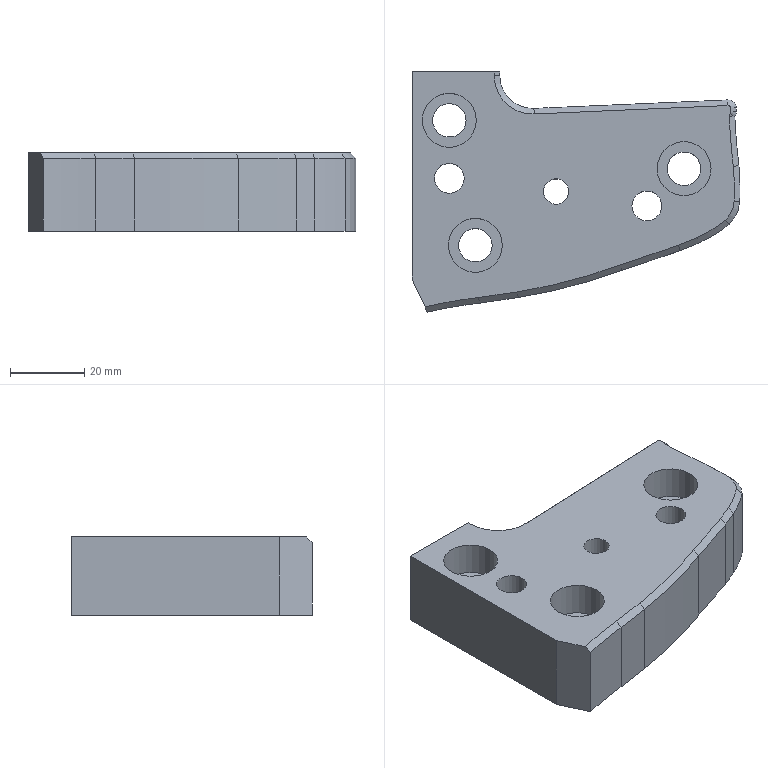Part | NX | features 23 2 | 1 solid | 48 faces | box 88.04 x 64.484 x 21 mm | volume 80340 mm3 | cylinder 20 | plane 16 | cone 12 | commonest cylinder face diameters 9 x3 14.5 x3 4.4 x2 8.001 x2 6.8 x1 17.6 x1
STEP:
#1=CARTESIAN_POINT('',(1059.999,248.439,-23.5));
#2=VERTEX_POINT('',#1);
#3=CARTESIAN_POINT('',(1064.,248.439,-23.5));
#4=DIRECTION('',(0.,0.,1.));
#5=DIRECTION('',(-1.,0.,0.));
#6=AXIS2_PLACEMENT_3D('',#3,#4,#5);
#7=CIRCLE('',#6,4.);
#8=EDGE_CURVE('',#2,#2,#7,.T.);
#9=ORIENTED_EDGE('',*,*,#8,.T.);
#10=EDGE_LOOP('',(#9));
#11=FACE_BOUND('',#10,.T.);
#12=CARTESIAN_POINT('',(1059.5,264.,-23.5));
#13=VERTEX_POINT('',#12);
#14=CARTESIAN_POINT('',(1064.,264.,-23.5));
#15=DIRECTION('',(0.,0.,1.));
#16=DIRECTION('',(-1.,0.,0.));
#17=AXIS2_PLACEMENT_3D('',#14,#15,#16);
#18=CIRCLE('',#17,4.5);
#19=EDGE_CURVE('',#13,#13,#18,.T.);
#20=ORIENTED_EDGE('',*,*,#19,.T.);
#21=EDGE_LOOP('',(#20));
#22=FACE_BOUND('',#21,.T.);
#23=CARTESIAN_POINT('',(1122.54,251.,-23.5));
#24=VERTEX_POINT('',#23);
#25=CARTESIAN_POINT('',(1127.04,251.,-23.5));
#26=DIRECTION('',(0.,0.,1.));
#27=DIRECTION('',(-1.,0.,0.));
#28=AXIS2_PLACEMENT_3D('',#25,#26,#27);
#29=CIRCLE('',#28,4.5);
#30=EDGE_CURVE('',#24,#24,#29,.T.);
#31=ORIENTED_EDGE('',*,*,#30,.T.);
#32=EDGE_LOOP('',(#31));
#33=FACE_BOUND('',#32,.T.);
#34=CARTESIAN_POINT('',(1066.5,230.439,-23.5));
#35=VERTEX_POINT('',#34);
#36=CARTESIAN_POINT('',(1071.,230.439,-23.5));
#37=DIRECTION('',(0.,0.,1.));
#38=DIRECTION('',(-1.,0.,0.));
#39=AXIS2_PLACEMENT_3D('',#36,#37,#38);
#40=CIRCLE('',#39,4.5);
#41=EDGE_CURVE('',#35,#35,#40,.T.);
#42=ORIENTED_EDGE('',*,*,#41,.T.);
#43=EDGE_LOOP('',(#42));
#44=FACE_BOUND('',#43,.T.);
#45=CARTESIAN_POINT('',(1113.04,241.,-23.5));
#46=VERTEX_POINT('',#45);
#47=CARTESIAN_POINT('',(1117.04,241.,-23.5));
#48=DIRECTION('',(0.,0.,1.));
#49=DIRECTION('',(-1.,0.,0.));
#50=AXIS2_PLACEMENT_3D('',#47,#48,#49);
#51=CIRCLE('',#50,4.);
#52=EDGE_CURVE('',#46,#46,#51,.T.);
#53=ORIENTED_EDGE('',*,*,#52,.T.);
#54=EDGE_LOOP('',(#53));
#55=FACE_BOUND('',#54,.T.);
#56=CARTESIAN_POINT('',(1089.301,244.877,-23.5));
#57=VERTEX_POINT('',#56);
#58=CARTESIAN_POINT('',(1092.701,244.877,-23.5));
#59=DIRECTION('',(0.,0.,1.));
#60=DIRECTION('',(-1.,0.,0.));
#61=AXIS2_PLACEMENT_3D('',#58,#59,#60);
#62=CIRCLE('',#61,3.4);
#63=EDGE_CURVE('',#57,#57,#62,.T.);
#64=ORIENTED_EDGE('',*,*,#63,.T.);
#65=EDGE_LOOP('',(#64));
#66=FACE_BOUND('',#65,.T.);
#67=CARTESIAN_POINT('',(1058.121,212.516,-23.5));
#68=VERTEX_POINT('',#67);
#69=CARTESIAN_POINT('',(1072.065,214.923,-23.5));
#70=VERTEX_POINT('',#69);
#71=CARTESIAN_POINT('',(1086.33,90.693,-23.5));
#72=DIRECTION('',(0.,0.,-1.));
#73=DIRECTION('',(-1.,0.,0.));
#74=AXIS2_PLACEMENT_3D('',#71,#72,#73);
#75=CIRCLE('',#74,125.047);
#76=EDGE_CURVE('',#68,#70,#75,.T.);
#77=ORIENTED_EDGE('',*,*,#76,.F.);
#78=CARTESIAN_POINT('',(1054.,221.377,-23.5));
#79=VERTEX_POINT('',#78);
#80=CARTESIAN_POINT('',(1052.952,223.63,-23.5));
#81=DIRECTION('',(0.4218,-0.9067,0.));
#82=VECTOR('',#81,1000.);
#83=LINE('',#80,#82);
#84=EDGE_CURVE('',#79,#68,#83,.T.);
#85=ORIENTED_EDGE('',*,*,#84,.F.);
#86=CARTESIAN_POINT('',(1054.,277.,-23.5));
#87=VERTEX_POINT('',#86);
#88=CARTESIAN_POINT('',(1054.,328.5,-23.5));
#89=DIRECTION('',(0.,1.,0.));
#90=VECTOR('',#89,1000.);
#91=LINE('',#88,#90);
#92=EDGE_CURVE('',#79,#87,#91,.T.);
#93=ORIENTED_EDGE('',*,*,#92,.T.);
#94=CARTESIAN_POINT('',(1077.541,277.,-23.5));
#95=VERTEX_POINT('',#94);
#96=CARTESIAN_POINT('',(1136.,277.,-23.5));
#97=DIRECTION('',(1.,0.,0.));
#98=VECTOR('',#97,1000.);
#99=LINE('',#96,#98);
#100=EDGE_CURVE('',#87,#95,#99,.T.);
#101=ORIENTED_EDGE('',*,*,#100,.T.);
#102=CARTESIAN_POINT('',(1077.541,275.983,-23.5));
#103=VERTEX_POINT('',#102);
#104=CARTESIAN_POINT('',(1077.541,328.5,-23.5));
#105=DIRECTION('',(0.,-1.,0.));
#106=VECTOR('',#105,1000.);
#107=LINE('',#104,#106);
#108=EDGE_CURVE('',#95,#103,#107,.T.);
#109=ORIENTED_EDGE('',*,*,#108,.T.);
#110=CARTESIAN_POINT('',(1086.725,267.191,-23.5));
#111=VERTEX_POINT('',#110);
#112=CARTESIAN_POINT('',(1086.341,275.983,-23.5));
#113=DIRECTION('',(0.,0.,1.));
#114=DIRECTION('',(-1.,0.,0.));
#115=AXIS2_PLACEMENT_3D('',#112,#113,#114);
#116=CIRCLE('',#115,8.8);
#117=EDGE_CURVE('',#103,#111,#116,.T.);
#118=ORIENTED_EDGE('',*,*,#117,.T.);
#119=CARTESIAN_POINT('',(1138.773,269.461,-23.5));
#120=VERTEX_POINT('',#119);
#121=CARTESIAN_POINT('',(1138.575,269.452,-23.5));
#122=DIRECTION('',(0.9991,0.04356,0.));
#123=VECTOR('',#122,1000.);
#124=LINE('',#121,#123);
#125=EDGE_CURVE('',#111,#120,#124,.T.);
#126=ORIENTED_EDGE('',*,*,#125,.T.);
#127=CARTESIAN_POINT('',(1141.067,267.339,-23.5));
#128=VERTEX_POINT('',#127);
#129=CARTESIAN_POINT('',(1138.868,267.263,-23.5));
#130=DIRECTION('',(0.,0.,1.));
#131=DIRECTION('',(-1.,0.,0.));
#132=AXIS2_PLACEMENT_3D('',#129,#130,#131);
#133=CIRCLE('',#132,2.2);
#134=EDGE_CURVE('',#128,#120,#133,.T.);
#135=ORIENTED_EDGE('',*,*,#134,.F.);
#136=CARTESIAN_POINT('',(1141.104,266.344,-23.5));
#137=VERTEX_POINT('',#136);
#138=CARTESIAN_POINT('',(1326.856,273.811,-23.5));
#139=DIRECTION('',(0.,0.,1.));
#140=DIRECTION('',(-1.,0.,0.));
#141=AXIS2_PLACEMENT_3D('',#138,#139,#140);
#142=CIRCLE('',#141,185.901);
#143=EDGE_CURVE('',#128,#137,#142,.T.);
#144=ORIENTED_EDGE('',*,*,#143,.T.);
#145=CARTESIAN_POINT('',(1140.666,264.943,-23.5));
#146=VERTEX_POINT('',#145);
#147=CARTESIAN_POINT('',(1138.906,266.263,-23.5));
#148=DIRECTION('',(0.,0.,1.));
#149=DIRECTION('',(-1.,0.,0.));
#150=AXIS2_PLACEMENT_3D('',#147,#148,#149);
#151=CIRCLE('',#150,2.2);
#152=EDGE_CURVE('',#146,#137,#151,.T.);
#153=ORIENTED_EDGE('',*,*,#152,.F.);
#154=CARTESIAN_POINT('',(1141.757,251.812,-23.5));
#155=VERTEX_POINT('',#154);
#156=CARTESIAN_POINT('',(1326.856,273.811,-23.5));
#157=DIRECTION('',(0.,0.,1.));
#158=DIRECTION('',(-1.,0.,0.));
#159=AXIS2_PLACEMENT_3D('',#156,#157,#158);
#160=CIRCLE('',#159,186.401);
#161=EDGE_CURVE('',#146,#155,#160,.T.);
#162=ORIENTED_EDGE('',*,*,#161,.T.);
#163=CARTESIAN_POINT('',(1141.998,242.228,-23.5));
#164=VERTEX_POINT('',#163);
#165=CARTESIAN_POINT('',(1057.602,244.9,-23.5));
#166=DIRECTION('',(0.,0.,-1.));
#167=DIRECTION('',(-1.,0.,0.));
#168=AXIS2_PLACEMENT_3D('',#165,#166,#167);
#169=CIRCLE('',#168,84.438);
#170=EDGE_CURVE('',#155,#164,#169,.T.);
#171=ORIENTED_EDGE('',*,*,#170,.T.);
#172=CARTESIAN_POINT('',(1139.107,236.023,-23.5));
#173=VERTEX_POINT('',#172);
#174=CARTESIAN_POINT('',(1132.519,242.868,-23.5));
#175=DIRECTION('',(0.,0.,1.));
#176=DIRECTION('',(-1.,0.,0.));
#177=AXIS2_PLACEMENT_3D('',#174,#175,#176);
#178=CIRCLE('',#177,9.5);
#179=EDGE_CURVE('',#173,#164,#178,.T.);
#180=ORIENTED_EDGE('',*,*,#179,.F.);
#181=CARTESIAN_POINT('',(1131.001,231.048,-23.5));
#182=VERTEX_POINT('',#181);
#183=CARTESIAN_POINT('',(1115.023,266.175,-23.5));
#184=DIRECTION('',(0.,0.,-1.));
#185=DIRECTION('',(-1.,0.,0.));
#186=AXIS2_PLACEMENT_3D('',#183,#184,#185);
#187=CIRCLE('',#186,38.59);
#188=EDGE_CURVE('',#173,#182,#187,.T.);
#189=ORIENTED_EDGE('',*,*,#188,.T.);
#190=CARTESIAN_POINT('',(1126.024,229.046,-23.5));
#191=VERTEX_POINT('',#190);
#192=CARTESIAN_POINT('',(1169.044,246.35,-23.5));
#193=DIRECTION('',(0.9278,0.3732,0.));
#194=VECTOR('',#193,1000.);
#195=LINE('',#192,#194);
#196=EDGE_CURVE('',#191,#182,#195,.T.);
#197=ORIENTED_EDGE('',*,*,#196,.F.);
#198=CARTESIAN_POINT('',(1110.455,223.763,-23.5));
#199=VERTEX_POINT('',#198);
#200=CARTESIAN_POINT('',(597.176,1761.975,-23.5));
#201=DIRECTION('',(0.,0.,1.));
#202=DIRECTION('',(-1.,0.,0.));
#203=AXIS2_PLACEMENT_3D('',#200,#201,#202);
#204=CIRCLE('',#203,1621.589);
#205=EDGE_CURVE('',#199,#191,#204,.T.);
#206=ORIENTED_EDGE('',*,*,#205,.F.);
#207=CARTESIAN_POINT('',(1082.518,216.438,-23.5));
#208=VERTEX_POINT('',#207);
#209=CARTESIAN_POINT('',(1058.804,363.809,-23.5));
#210=DIRECTION('',(0.,0.,1.));
#211=DIRECTION('',(-1.,0.,0.));
#212=AXIS2_PLACEMENT_3D('',#209,#210,#211);
#213=CIRCLE('',#212,149.267);
#214=EDGE_CURVE('',#208,#199,#213,.T.);
#215=ORIENTED_EDGE('',*,*,#214,.F.);
#216=CARTESIAN_POINT('',(1087.282,217.128,-23.5));
#217=DIRECTION('',(-0.9897,-0.1434,0.));
#218=VECTOR('',#217,1000.);
#219=LINE('',#216,#218);
#220=EDGE_CURVE('',#208,#70,#219,.T.);
#221=ORIENTED_EDGE('',*,*,#220,.T.);
#222=EDGE_LOOP('',(#77,#85,#93,#101,#109,#118,#126,#135,#144,#153,#162,#171,#180,#189,#197,#206,#215,#221));
#223=FACE_BOUND('',#222,.T.);
#224=CARTESIAN_POINT('',(1136.,328.5,-23.5));
#225=DIRECTION('',(0.,0.,-1.));
#226=DIRECTION('',(1.,0.,0.));
#227=AXIS2_PLACEMENT_3D('',#224,#225,#226);
#228=PLANE('',#227);
#229=ADVANCED_FACE('',(#11,#22,#33,#44,#55,#66,#223),#228,.T.);
#230=CARTESIAN_POINT('',(1054.,221.377,-2.5));
#231=VERTEX_POINT('',#230);
#232=CARTESIAN_POINT('',(1057.475,213.906,-2.5));
#233=VERTEX_POINT('',#232);
#234=CARTESIAN_POINT('',(1051.784,226.14,-2.5));
#235=DIRECTION('',(0.4218,-0.9067,0.));
#236=VECTOR('',#235,1000.);
#237=LINE('',#234,#236);
#238=EDGE_CURVE('',#231,#233,#237,.T.);
#239=ORIENTED_EDGE('',*,*,#238,.T.);
#240=CARTESIAN_POINT('',(1071.872,216.411,-2.5));
#241=VERTEX_POINT('',#240);
#242=CARTESIAN_POINT('',(1086.33,90.693,-2.5));
#243=DIRECTION('',(0.,0.,1.));
#244=DIRECTION('',(1.,0.,0.));
#245=AXIS2_PLACEMENT_3D('',#242,#243,#244);
#246=CIRCLE('',#245,126.547);
#247=EDGE_CURVE('',#241,#233,#246,.T.);
#248=ORIENTED_EDGE('',*,*,#247,.F.);
#249=CARTESIAN_POINT('',(1082.291,217.921,-2.5));
#250=VERTEX_POINT('',#249);
#251=CARTESIAN_POINT('',(1478.441,275.317,-2.5));
#252=DIRECTION('',(0.9897,0.1434,0.));
#253=VECTOR('',#252,1000.);
#254=LINE('',#251,#253);
#255=EDGE_CURVE('',#241,#250,#254,.T.);
#256=ORIENTED_EDGE('',*,*,#255,.T.);
#257=CARTESIAN_POINT('',(1109.958,225.179,-2.5));
#258=VERTEX_POINT('',#257);
#259=CARTESIAN_POINT('',(1058.804,363.809,-2.5));
#260=DIRECTION('',(0.,0.,1.));
#261=DIRECTION('',(1.,0.,0.));
#262=AXIS2_PLACEMENT_3D('',#259,#260,#261);
#263=CIRCLE('',#262,147.767);
#264=EDGE_CURVE('',#250,#258,#263,.T.);
#265=ORIENTED_EDGE('',*,*,#264,.T.);
#266=CARTESIAN_POINT('',(1125.499,230.452,-2.5));
#267=VERTEX_POINT('',#266);
#268=CARTESIAN_POINT('',(597.176,1761.975,-2.5));
#269=DIRECTION('',(0.,0.,1.));
#270=DIRECTION('',(1.,0.,0.));
#271=AXIS2_PLACEMENT_3D('',#268,#269,#270);
#272=CIRCLE('',#271,1620.089);
#273=EDGE_CURVE('',#258,#267,#272,.T.);
#274=ORIENTED_EDGE('',*,*,#273,.T.);
#275=CARTESIAN_POINT('',(1130.41,232.427,-2.5));
#276=VERTEX_POINT('',#275);
#277=CARTESIAN_POINT('',(1289.696,296.498,-2.5));
#278=DIRECTION('',(0.9278,0.3732,0.));
#279=VECTOR('',#278,1000.);
#280=LINE('',#277,#279);
#281=EDGE_CURVE('',#267,#276,#280,.T.);
#282=ORIENTED_EDGE('',*,*,#281,.T.);
#283=CARTESIAN_POINT('',(1138.115,237.15,-2.5));
#284=VERTEX_POINT('',#283);
#285=CARTESIAN_POINT('',(1115.023,266.175,-2.5));
#286=DIRECTION('',(0.,0.,1.));
#287=DIRECTION('',(1.,0.,0.));
#288=AXIS2_PLACEMENT_3D('',#285,#286,#287);
#289=CIRCLE('',#288,37.09);
#290=EDGE_CURVE('',#276,#284,#289,.T.);
#291=ORIENTED_EDGE('',*,*,#290,.T.);
#292=CARTESIAN_POINT('',(1140.5,242.304,-2.5));
#293=VERTEX_POINT('',#292);
#294=CARTESIAN_POINT('',(1132.519,242.868,-2.5));
#295=DIRECTION('',(0.,0.,1.));
#296=DIRECTION('',(1.,0.,0.));
#297=AXIS2_PLACEMENT_3D('',#294,#295,#296);
#298=CIRCLE('',#297,8.);
#299=EDGE_CURVE('',#284,#293,#298,.T.);
#300=ORIENTED_EDGE('',*,*,#299,.T.);
#301=CARTESIAN_POINT('',(1140.264,251.662,-2.5));
#302=VERTEX_POINT('',#301);
#303=CARTESIAN_POINT('',(1057.602,244.9,-2.5));
#304=DIRECTION('',(0.,0.,1.));
#305=DIRECTION('',(1.,0.,0.));
#306=AXIS2_PLACEMENT_3D('',#303,#304,#305);
#307=CIRCLE('',#306,82.938);
#308=EDGE_CURVE('',#293,#302,#307,.T.);
#309=ORIENTED_EDGE('',*,*,#308,.T.);
#310=CARTESIAN_POINT('',(1139.164,264.946,-2.5));
#311=VERTEX_POINT('',#310);
#312=CARTESIAN_POINT('',(1326.856,273.811,-2.5));
#313=DIRECTION('',(0.,0.,1.));
#314=DIRECTION('',(1.,0.,0.));
#315=AXIS2_PLACEMENT_3D('',#312,#313,#314);
#316=CIRCLE('',#315,187.901);
#317=EDGE_CURVE('',#311,#302,#316,.T.);
#318=ORIENTED_EDGE('',*,*,#317,.F.);
#319=CARTESIAN_POINT('',(1139.451,265.824,-2.5));
#320=VERTEX_POINT('',#319);
#321=CARTESIAN_POINT('',(1140.462,265.007,-2.5));
#322=DIRECTION('',(0.,0.,1.));
#323=DIRECTION('',(1.,0.,0.));
#324=AXIS2_PLACEMENT_3D('',#321,#322,#323);
#325=CIRCLE('',#324,1.3);
#326=EDGE_CURVE('',#320,#311,#325,.T.);
#327=ORIENTED_EDGE('',*,*,#326,.F.);
#328=CARTESIAN_POINT('',(1139.606,266.287,-2.5));
#329=VERTEX_POINT('',#328);
#330=CARTESIAN_POINT('',(1138.906,266.263,-2.5));
#331=DIRECTION('',(0.,0.,1.));
#332=DIRECTION('',(1.,0.,0.));
#333=AXIS2_PLACEMENT_3D('',#330,#331,#332);
#334=CIRCLE('',#333,0.7);
#335=EDGE_CURVE('',#320,#329,#334,.T.);
#336=ORIENTED_EDGE('',*,*,#335,.T.);
#337=CARTESIAN_POINT('',(1139.568,267.287,-2.5));
#338=VERTEX_POINT('',#337);
#339=CARTESIAN_POINT('',(1326.856,273.811,-2.5));
#340=DIRECTION('',(0.,0.,1.));
#341=DIRECTION('',(1.,0.,0.));
#342=AXIS2_PLACEMENT_3D('',#339,#340,#341);
#343=CIRCLE('',#342,187.401);
#344=EDGE_CURVE('',#338,#329,#343,.T.);
#345=ORIENTED_EDGE('',*,*,#344,.F.);
#346=CARTESIAN_POINT('',(1138.838,267.962,-2.5));
#347=VERTEX_POINT('',#346);
#348=CARTESIAN_POINT('',(1138.868,267.263,-2.5));
#349=DIRECTION('',(0.,0.,1.));
#350=DIRECTION('',(1.,0.,0.));
#351=AXIS2_PLACEMENT_3D('',#348,#349,#350);
#352=CIRCLE('',#351,0.7);
#353=EDGE_CURVE('',#338,#347,#352,.T.);
#354=ORIENTED_EDGE('',*,*,#353,.T.);
#355=CARTESIAN_POINT('',(1086.79,265.693,-2.5));
#356=VERTEX_POINT('',#355);
#357=CARTESIAN_POINT('',(1548.912,285.843,-2.5));
#358=DIRECTION('',(-0.9991,-0.04356,0.));
#359=VECTOR('',#358,1000.);
#360=LINE('',#357,#359);
#361=EDGE_CURVE('',#347,#356,#360,.T.);
#362=ORIENTED_EDGE('',*,*,#361,.T.);
#363=CARTESIAN_POINT('',(1076.041,275.983,-2.5));
#364=VERTEX_POINT('',#363);
#365=CARTESIAN_POINT('',(1086.341,275.983,-2.5));
#366=DIRECTION('',(0.,0.,1.));
#367=DIRECTION('',(1.,0.,0.));
#368=AXIS2_PLACEMENT_3D('',#365,#366,#367);
#369=CIRCLE('',#368,10.3);
#370=EDGE_CURVE('',#364,#356,#369,.T.);
#371=ORIENTED_EDGE('',*,*,#370,.F.);
#372=CARTESIAN_POINT('',(1076.041,277.,-2.5));
#373=VERTEX_POINT('',#372);
#374=CARTESIAN_POINT('',(1076.041,-425.,-2.5));
#375=DIRECTION('',(0.,1.,0.));
#376=VECTOR('',#375,1000.);
#377=LINE('',#374,#376);
#378=EDGE_CURVE('',#364,#373,#377,.T.);
#379=ORIENTED_EDGE('',*,*,#378,.T.);
#380=CARTESIAN_POINT('',(1054.,277.,-2.5));
#381=VERTEX_POINT('',#380);
#382=CARTESIAN_POINT('',(1166.5,277.,-2.5));
#383=DIRECTION('',(-1.,0.,0.));
#384=VECTOR('',#383,1000.);
#385=LINE('',#382,#384);
#386=EDGE_CURVE('',#373,#381,#385,.T.);
#387=ORIENTED_EDGE('',*,*,#386,.T.);
#388=CARTESIAN_POINT('',(1054.,328.5,-2.5));
#389=DIRECTION('',(0.,-1.,0.));
#390=VECTOR('',#389,1000.);
#391=LINE('',#388,#390);
#392=EDGE_CURVE('',#381,#231,#391,.T.);
#393=ORIENTED_EDGE('',*,*,#392,.T.);
#394=EDGE_LOOP('',(#239,#248,#256,#265,#274,#282,#291,#300,#309,#318,#327,#336,#345,#354,#362,#371,#379,#387,#393));
#395=FACE_BOUND('',#394,.T.);
#396=CARTESIAN_POINT('',(1068.001,248.439,-2.5));
#397=VERTEX_POINT('',#396);
#398=CARTESIAN_POINT('',(1064.,248.439,-2.5));
#399=DIRECTION('',(0.,0.,-1.));
#400=DIRECTION('',(1.,0.,0.));
#401=AXIS2_PLACEMENT_3D('',#398,#399,#400);
#402=CIRCLE('',#401,4.);
#403=EDGE_CURVE('',#397,#397,#402,.T.);
#404=ORIENTED_EDGE('',*,*,#403,.T.);
#405=EDGE_LOOP('',(#404));
#406=FACE_BOUND('',#405,.T.);
#407=CARTESIAN_POINT('',(1071.25,264.,-2.5));
#408=VERTEX_POINT('',#407);
#409=CARTESIAN_POINT('',(1064.,264.,-2.5));
#410=DIRECTION('',(0.,0.,-1.));
#411=DIRECTION('',(1.,0.,0.));
#412=AXIS2_PLACEMENT_3D('',#409,#410,#411);
#413=CIRCLE('',#412,7.25);
#414=EDGE_CURVE('',#408,#408,#413,.T.);
#415=ORIENTED_EDGE('',*,*,#414,.T.);
#416=EDGE_LOOP('',(#415));
#417=FACE_BOUND('',#416,.T.);
#418=CARTESIAN_POINT('',(1134.29,251.,-2.5));
#419=VERTEX_POINT('',#418);
#420=CARTESIAN_POINT('',(1127.04,251.,-2.5));
#421=DIRECTION('',(0.,0.,-1.));
#422=DIRECTION('',(1.,0.,0.));
#423=AXIS2_PLACEMENT_3D('',#420,#421,#422);
#424=CIRCLE('',#423,7.25);
#425=EDGE_CURVE('',#419,#419,#424,.T.);
#426=ORIENTED_EDGE('',*,*,#425,.T.);
#427=EDGE_LOOP('',(#426));
#428=FACE_BOUND('',#427,.T.);
#429=CARTESIAN_POINT('',(1078.25,230.439,-2.5));
#430=VERTEX_POINT('',#429);
#431=CARTESIAN_POINT('',(1071.,230.439,-2.5));
#432=DIRECTION('',(0.,0.,-1.));
#433=DIRECTION('',(1.,0.,0.));
#434=AXIS2_PLACEMENT_3D('',#431,#432,#433);
#435=CIRCLE('',#434,7.25);
#436=EDGE_CURVE('',#430,#430,#435,.T.);
#437=ORIENTED_EDGE('',*,*,#436,.T.);
#438=EDGE_LOOP('',(#437));
#439=FACE_BOUND('',#438,.T.);
#440=CARTESIAN_POINT('',(1121.041,241.,-2.5));
#441=VERTEX_POINT('',#440);
#442=CARTESIAN_POINT('',(1117.04,241.,-2.5));
#443=DIRECTION('',(0.,0.,-1.));
#444=DIRECTION('',(1.,0.,0.));
#445=AXIS2_PLACEMENT_3D('',#442,#443,#444);
#446=CIRCLE('',#445,4.);
#447=EDGE_CURVE('',#441,#441,#446,.T.);
#448=ORIENTED_EDGE('',*,*,#447,.T.);
#449=EDGE_LOOP('',(#448));
#450=FACE_BOUND('',#449,.T.);
#451=CARTESIAN_POINT('',(1096.101,244.877,-2.5));
#452=VERTEX_POINT('',#451);
#453=CARTESIAN_POINT('',(1092.701,244.877,-2.5));
#454=DIRECTION('',(0.,0.,1.));
#455=DIRECTION('',(1.,0.,0.));
#456=AXIS2_PLACEMENT_3D('',#453,#454,#455);
#457=CIRCLE('',#456,3.4);
#458=EDGE_CURVE('',#452,#452,#457,.T.);
#459=ORIENTED_EDGE('',*,*,#458,.F.);
#460=EDGE_LOOP('',(#459));
#461=FACE_BOUND('',#460,.T.);
#462=CARTESIAN_POINT('',(1166.5,279.5,-2.5));
#463=DIRECTION('',(0.,0.,1.));
#464=DIRECTION('',(-1.,0.,0.));
#465=AXIS2_PLACEMENT_3D('',#462,#463,#464);
#466=PLANE('',#465);
#467=ADVANCED_FACE('',(#395,#406,#417,#428,#439,#450,#461),#466,.T.);
#468=ORIENTED_EDGE('',*,*,#326,.T.);
#469=CARTESIAN_POINT('',(1140.462,265.007,-3.8));
#470=VERTEX_POINT('',#469);
#471=CARTESIAN_POINT('',(1140.163,264.993,-3.5));
#472=DIRECTION('',(-0.7063,-0.03336,0.7071));
#473=VECTOR('',#472,1000.);
#474=LINE('',#471,#473);
#475=EDGE_CURVE('',#470,#311,#474,.T.);
#476=ORIENTED_EDGE('',*,*,#475,.F.);
#477=CARTESIAN_POINT('',(1140.229,265.196,-3.5));
#478=DIRECTION('',(-0.5502,0.4441,0.7071));
#479=VECTOR('',#478,1000.);
#480=LINE('',#477,#479);
#481=EDGE_CURVE('',#470,#320,#480,.T.);
#482=ORIENTED_EDGE('',*,*,#481,.T.);
#483=EDGE_LOOP('',(#468,#476,#482));
#484=FACE_BOUND('',#483,.T.);
#485=CARTESIAN_POINT('',(1140.462,265.007,-3.5));
#486=DIRECTION('',(0.,0.,1.));
#487=DIRECTION('',(1.,0.,0.));
#488=AXIS2_PLACEMENT_3D('',#485,#486,#487);
#489=CONICAL_SURFACE('',#488,0.3,0.7854);
#490=ADVANCED_FACE('',(#484),#489,.F.);
#491=CARTESIAN_POINT('',(1138.773,269.461,-4.));
#492=VERTEX_POINT('',#491);
#493=CARTESIAN_POINT('',(1086.725,267.191,-4.));
#494=VERTEX_POINT('',#493);
#495=CARTESIAN_POINT('',(1585.84,288.955,-4.));
#496=DIRECTION('',(-0.9991,-0.04356,0.));
#497=VECTOR('',#496,1000.);
#498=LINE('',#495,#497);
#499=EDGE_CURVE('',#492,#494,#498,.T.);
#500=ORIENTED_EDGE('',*,*,#499,.T.);
#501=CARTESIAN_POINT('',(1086.746,266.692,-3.5));
#502=DIRECTION('',(0.0308,-0.7064,0.7071));
#503=VECTOR('',#502,1000.);
#504=LINE('',#501,#503);
#505=EDGE_CURVE('',#494,#356,#504,.T.);
#506=ORIENTED_EDGE('',*,*,#505,.T.);
#507=ORIENTED_EDGE('',*,*,#361,.F.);
#508=CARTESIAN_POINT('',(1138.794,268.961,-3.5));
#509=DIRECTION('',(0.0308,-0.7064,0.7071));
#510=VECTOR('',#509,1000.);
#511=LINE('',#508,#510);
#512=EDGE_CURVE('',#492,#347,#511,.T.);
#513=ORIENTED_EDGE('',*,*,#512,.F.);
#514=EDGE_LOOP('',(#500,#506,#507,#513));
#515=FACE_BOUND('',#514,.T.);
#516=CARTESIAN_POINT('',(1548.868,286.842,-3.5));
#517=DIRECTION('',(-0.0308,0.7064,0.7071));
#518=DIRECTION('',(0.9991,0.04356,0.));
#519=AXIS2_PLACEMENT_3D('',#516,#517,#518);
#520=PLANE('',#519);
#521=ADVANCED_FACE('',(#515),#520,.T.);
#522=ORIENTED_EDGE('',*,*,#512,.T.);
#523=ORIENTED_EDGE('',*,*,#353,.F.);
#524=CARTESIAN_POINT('',(1141.067,267.339,-4.));
#525=VERTEX_POINT('',#524);
#526=CARTESIAN_POINT('',(1140.567,267.322,-3.5));
#527=DIRECTION('',(-0.7067,-0.02462,0.7071));
#528=VECTOR('',#527,1000.);
#529=LINE('',#526,#528);
#530=EDGE_CURVE('',#525,#338,#529,.T.);
#531=ORIENTED_EDGE('',*,*,#530,.F.);
#532=CARTESIAN_POINT('',(1138.868,267.263,-4.));
#533=DIRECTION('',(0.,0.,1.));
#534=DIRECTION('',(-1.,0.,0.));
#535=AXIS2_PLACEMENT_3D('',#532,#533,#534);
#536=CIRCLE('',#535,2.2);
#537=EDGE_CURVE('',#525,#492,#536,.T.);
#538=ORIENTED_EDGE('',*,*,#537,.T.);
#539=EDGE_LOOP('',(#522,#523,#531,#538));
#540=FACE_BOUND('',#539,.T.);
#541=CARTESIAN_POINT('',(1138.868,267.263,-3.5));
#542=DIRECTION('',(0.,0.,-1.));
#543=DIRECTION('',(-1.,0.,0.));
#544=AXIS2_PLACEMENT_3D('',#541,#542,#543);
#545=CONICAL_SURFACE('',#544,1.7,0.7854);
#546=ADVANCED_FACE('',(#540),#545,.T.);
#547=ORIENTED_EDGE('',*,*,#344,.T.);
#548=CARTESIAN_POINT('',(1141.104,266.344,-4.));
#549=VERTEX_POINT('',#548);
#550=CARTESIAN_POINT('',(1141.254,266.349,-4.15));
#551=CARTESIAN_POINT('',(1141.177,266.347,-4.073));
#552=CARTESIAN_POINT('',(1141.1,266.344,-3.996));
#553=CARTESIAN_POINT('',(1140.964,266.338,-3.86));
#554=CARTESIAN_POINT('',(1140.905,266.336,-3.801));
#555=CARTESIAN_POINT('',(1140.801,266.332,-3.696));
#556=CARTESIAN_POINT('',(1140.755,266.33,-3.651));
#557=CARTESIAN_POINT('',(1140.675,266.327,-3.57));
#558=CARTESIAN_POINT('',(1140.64,266.326,-3.535));
#559=CARTESIAN_POINT('',(1140.372,266.316,-3.267));
#560=CARTESIAN_POINT('',(1140.138,266.307,-3.033));
#561=CARTESIAN_POINT('',(1139.87,266.297,-2.765));
#562=CARTESIAN_POINT('',(1139.835,266.296,-2.73));
#563=CARTESIAN_POINT('',(1139.755,266.293,-2.65));
#564=CARTESIAN_POINT('',(1139.709,266.291,-2.604));
#565=CARTESIAN_POINT('',(1139.605,266.287,-2.499));
#566=CARTESIAN_POINT('',(1139.546,266.285,-2.44));
#567=CARTESIAN_POINT('',(1139.41,266.28,-2.304));
#568=CARTESIAN_POINT('',(1139.333,266.277,-2.227));
#569=CARTESIAN_POINT('',(1139.256,266.274,-2.15));
#570=B_SPLINE_CURVE_WITH_KNOTS('',3,(#550,#551,#552,#553,#554,#555,#556,#557,#558,#559,#560,#561,#562,#563,#564,#565,#566,#567,#568,#569),.UNSPECIFIED.,.F.,.F.,(4,2,2,2,2,2,2,2,2,4),(0.,0.1154,0.2041,0.2724,0.3249,0.6751,0.7276,0.7959,0.8846,1.),.UNSPECIFIED.);
#571=EDGE_CURVE('',#549,#329,#570,.T.);
#572=ORIENTED_EDGE('',*,*,#571,.F.);
#573=CARTESIAN_POINT('',(1326.856,273.811,-4.));
#574=DIRECTION('',(0.,0.,-1.));
#575=DIRECTION('',(-1.,0.,0.));
#576=AXIS2_PLACEMENT_3D('',#573,#574,#575);
#577=CIRCLE('',#576,185.901);
#578=EDGE_CURVE('',#549,#525,#577,.T.);
#579=ORIENTED_EDGE('',*,*,#578,.T.);
#580=ORIENTED_EDGE('',*,*,#530,.T.);
#581=EDGE_LOOP('',(#547,#572,#579,#580));
#582=FACE_BOUND('',#581,.T.);
#583=CARTESIAN_POINT('',(1326.856,273.811,-3.5));
#584=DIRECTION('',(0.,0.,1.));
#585=DIRECTION('',(1.,0.,0.));
#586=AXIS2_PLACEMENT_3D('',#583,#584,#585);
#587=CONICAL_SURFACE('',#586,186.401,0.7854);
#588=ADVANCED_FACE('',(#582),#587,.F.);
#589=ORIENTED_EDGE('',*,*,#571,.T.);
#590=ORIENTED_EDGE('',*,*,#335,.F.);
#591=ORIENTED_EDGE('',*,*,#481,.F.);
#592=CARTESIAN_POINT('',(1140.666,264.943,-4.));
#593=VERTEX_POINT('',#592);
#594=CARTESIAN_POINT('',(1140.666,264.943,-4.));
#595=CARTESIAN_POINT('',(1140.598,264.964,-3.933));
#596=CARTESIAN_POINT('',(1140.53,264.985,-3.867));
#597=CARTESIAN_POINT('',(1140.462,265.007,-3.8));
#598=B_SPLINE_CURVE_WITH_KNOTS('',3,(#594,#595,#596,#597),.UNSPECIFIED.,.F.,.F.,(4,4),(0.,1.),.PIECEWISE_BEZIER_KNOTS.);
#599=EDGE_CURVE('',#593,#470,#598,.T.);
#600=ORIENTED_EDGE('',*,*,#599,.F.);
#601=CARTESIAN_POINT('',(1138.906,266.263,-4.));
#602=DIRECTION('',(0.,0.,1.));
#603=DIRECTION('',(-1.,0.,0.));
#604=AXIS2_PLACEMENT_3D('',#601,#602,#603);
#605=CIRCLE('',#604,2.2);
#606=EDGE_CURVE('',#593,#549,#605,.T.);
#607=ORIENTED_EDGE('',*,*,#606,.T.);
#608=EDGE_LOOP('',(#589,#590,#591,#600,#607));
#609=FACE_BOUND('',#608,.T.);
#610=CARTESIAN_POINT('',(1138.906,266.263,-3.5));
#611=DIRECTION('',(0.,0.,-1.));
#612=DIRECTION('',(-1.,0.,0.));
#613=AXIS2_PLACEMENT_3D('',#610,#611,#612);
#614=CONICAL_SURFACE('',#613,1.7,0.7854);
#615=ADVANCED_FACE('',(#609),#614,.T.);
#616=ORIENTED_EDGE('',*,*,#317,.T.);
#617=CARTESIAN_POINT('',(1141.757,251.812,-4.));
#618=VERTEX_POINT('',#617);
#619=CARTESIAN_POINT('',(1141.906,251.827,-4.15));
#620=CARTESIAN_POINT('',(1141.83,251.819,-4.073));
#621=CARTESIAN_POINT('',(1141.753,251.811,-3.996));
#622=CARTESIAN_POINT('',(1141.618,251.798,-3.86));
#623=CARTESIAN_POINT('',(1141.559,251.792,-3.801));
#624=CARTESIAN_POINT('',(1141.455,251.781,-3.696));
#625=CARTESIAN_POINT('',(1141.409,251.777,-3.651));
#626=CARTESIAN_POINT('',(1141.329,251.769,-3.57));
#627=CARTESIAN_POINT('',(1141.294,251.765,-3.535));
#628=CARTESIAN_POINT('',(1141.027,251.739,-3.267));
#629=CARTESIAN_POINT('',(1140.795,251.715,-3.033));
#630=CARTESIAN_POINT('',(1140.528,251.689,-2.765));
#631=CARTESIAN_POINT('',(1140.493,251.685,-2.73));
#632=CARTESIAN_POINT('',(1140.413,251.677,-2.65));
#633=CARTESIAN_POINT('',(1140.368,251.672,-2.604));
#634=CARTESIAN_POINT('',(1140.264,251.662,-2.499));
#635=CARTESIAN_POINT('',(1140.205,251.656,-2.44));
#636=CARTESIAN_POINT('',(1140.069,251.643,-2.304));
#637=CARTESIAN_POINT('',(1139.993,251.635,-2.227));
#638=CARTESIAN_POINT('',(1139.916,251.627,-2.15));
#639=B_SPLINE_CURVE_WITH_KNOTS('',3,(#619,#620,#621,#622,#623,#624,#625,#626,#627,#628,#629,#630,#631,#632,#633,#634,#635,#636,#637,#638),.UNSPECIFIED.,.F.,.F.,(4,2,2,2,2,2,2,2,2,4),(0.,0.1154,0.2041,0.2724,0.3249,0.6751,0.7276,0.7959,0.8846,1.),.UNSPECIFIED.);
#640=EDGE_CURVE('',#618,#302,#639,.T.);
#641=ORIENTED_EDGE('',*,*,#640,.F.);
#642=CARTESIAN_POINT('',(1326.856,273.811,-4.));
#643=DIRECTION('',(0.,0.,-1.));
#644=DIRECTION('',(-1.,0.,0.));
#645=AXIS2_PLACEMENT_3D('',#642,#643,#644);
#646=CIRCLE('',#645,186.401);
#647=EDGE_CURVE('',#618,#593,#646,.T.);
#648=ORIENTED_EDGE('',*,*,#647,.T.);
#649=ORIENTED_EDGE('',*,*,#599,.T.);
#650=ORIENTED_EDGE('',*,*,#475,.T.);
#651=EDGE_LOOP('',(#616,#641,#648,#649,#650));
#652=FACE_BOUND('',#651,.T.);
#653=CARTESIAN_POINT('',(1326.856,273.811,-3.5));
#654=DIRECTION('',(0.,0.,1.));
#655=DIRECTION('',(1.,0.,0.));
#656=AXIS2_PLACEMENT_3D('',#653,#654,#655);
#657=CONICAL_SURFACE('',#656,186.901,0.7854);
#658=ADVANCED_FACE('',(#652),#657,.F.);
#659=ORIENTED_EDGE('',*,*,#640,.T.);
#660=ORIENTED_EDGE('',*,*,#308,.F.);
#661=CARTESIAN_POINT('',(1141.998,242.228,-4.));
#662=VERTEX_POINT('',#661);
#663=CARTESIAN_POINT('',(1142.148,242.221,-4.15));
#664=CARTESIAN_POINT('',(1142.071,242.225,-4.073));
#665=CARTESIAN_POINT('',(1141.994,242.228,-3.996));
#666=CARTESIAN_POINT('',(1141.858,242.235,-3.86));
#667=CARTESIAN_POINT('',(1141.799,242.238,-3.801));
#668=CARTESIAN_POINT('',(1141.695,242.243,-3.696));
#669=CARTESIAN_POINT('',(1141.649,242.246,-3.651));
#670=CARTESIAN_POINT('',(1141.569,242.25,-3.57));
#671=CARTESIAN_POINT('',(1141.534,242.251,-3.535));
#672=CARTESIAN_POINT('',(1141.266,242.265,-3.267));
#673=CARTESIAN_POINT('',(1141.033,242.277,-3.033));
#674=CARTESIAN_POINT('',(1140.765,242.29,-2.765));
#675=CARTESIAN_POINT('',(1140.73,242.292,-2.73));
#676=CARTESIAN_POINT('',(1140.649,242.296,-2.65));
#677=CARTESIAN_POINT('',(1140.604,242.298,-2.604));
#678=CARTESIAN_POINT('',(1140.499,242.304,-2.499));
#679=CARTESIAN_POINT('',(1140.44,242.307,-2.44));
#680=CARTESIAN_POINT('',(1140.304,242.313,-2.304));
#681=CARTESIAN_POINT('',(1140.227,242.317,-2.227));
#682=CARTESIAN_POINT('',(1140.151,242.321,-2.15));
#683=B_SPLINE_CURVE_WITH_KNOTS('',3,(#663,#664,#665,#666,#667,#668,#669,#670,#671,#672,#673,#674,#675,#676,#677,#678,#679,#680,#681,#682),.UNSPECIFIED.,.F.,.F.,(4,2,2,2,2,2,2,2,2,4),(0.,0.1154,0.2041,0.2724,0.3249,0.6751,0.7276,0.7959,0.8846,1.),.UNSPECIFIED.);
#684=EDGE_CURVE('',#662,#293,#683,.T.);
#685=ORIENTED_EDGE('',*,*,#684,.F.);
#686=CARTESIAN_POINT('',(1057.602,244.9,-4.));
#687=DIRECTION('',(0.,0.,1.));
#688=DIRECTION('',(-1.,0.,0.));
#689=AXIS2_PLACEMENT_3D('',#686,#687,#688);
#690=CIRCLE('',#689,84.438);
#691=EDGE_CURVE('',#662,#618,#690,.T.);
#692=ORIENTED_EDGE('',*,*,#691,.T.);
#693=EDGE_LOOP('',(#659,#660,#685,#692));
#694=FACE_BOUND('',#693,.T.);
#695=CARTESIAN_POINT('',(1057.602,244.9,-3.5));
#696=DIRECTION('',(0.,0.,-1.));
#697=DIRECTION('',(-1.,0.,0.));
#698=AXIS2_PLACEMENT_3D('',#695,#696,#697);
#699=CONICAL_SURFACE('',#698,83.938,0.7854);
#700=ADVANCED_FACE('',(#694),#699,.T.);
#701=ORIENTED_EDGE('',*,*,#684,.T.);
#702=ORIENTED_EDGE('',*,*,#299,.F.);
#703=CARTESIAN_POINT('',(1139.107,236.023,-4.));
#704=VERTEX_POINT('',#703);
#705=CARTESIAN_POINT('',(1139.107,236.023,-4.));
#706=CARTESIAN_POINT('',(1138.997,236.148,-3.833));
#707=CARTESIAN_POINT('',(1138.887,236.274,-3.667));
#708=CARTESIAN_POINT('',(1138.556,236.65,-3.167));
#709=CARTESIAN_POINT('',(1138.336,236.9,-2.833));
#710=CARTESIAN_POINT('',(1138.115,237.15,-2.5));
#711=B_SPLINE_CURVE_WITH_KNOTS('',3,(#705,#706,#707,#708,#709,#710),.UNSPECIFIED.,.F.,.F.,(4,2,4),(0.,0.3333,1.),.UNSPECIFIED.);
#712=EDGE_CURVE('',#704,#284,#711,.T.);
#713=ORIENTED_EDGE('',*,*,#712,.F.);
#714=CARTESIAN_POINT('',(1132.519,242.868,-4.));
#715=DIRECTION('',(0.,0.,1.));
#716=DIRECTION('',(-1.,0.,0.));
#717=AXIS2_PLACEMENT_3D('',#714,#715,#716);
#718=CIRCLE('',#717,9.5);
#719=EDGE_CURVE('',#704,#662,#718,.T.);
#720=ORIENTED_EDGE('',*,*,#719,.T.);
#721=EDGE_LOOP('',(#701,#702,#713,#720));
#722=FACE_BOUND('',#721,.T.);
#723=CARTESIAN_POINT('',(1132.519,242.868,-3.5));
#724=DIRECTION('',(0.,0.,-1.));
#725=DIRECTION('',(-1.,0.,0.));
#726=AXIS2_PLACEMENT_3D('',#723,#724,#725);
#727=CONICAL_SURFACE('',#726,9.,0.7854);
#728=ADVANCED_FACE('',(#722),#727,.T.);
#729=ORIENTED_EDGE('',*,*,#712,.T.);
#730=ORIENTED_EDGE('',*,*,#290,.F.);
#731=CARTESIAN_POINT('',(1131.001,231.048,-4.));
#732=VERTEX_POINT('',#731);
#733=CARTESIAN_POINT('',(1131.06,230.911,-4.15));
#734=CARTESIAN_POINT('',(1131.03,230.981,-4.073));
#735=CARTESIAN_POINT('',(1130.999,231.052,-3.996));
#736=CARTESIAN_POINT('',(1130.946,231.177,-3.86));
#737=CARTESIAN_POINT('',(1130.922,231.231,-3.801));
#738=CARTESIAN_POINT('',(1130.881,231.328,-3.696));
#739=CARTESIAN_POINT('',(1130.863,231.369,-3.651));
#740=CARTESIAN_POINT('',(1130.832,231.443,-3.57));
#741=CARTESIAN_POINT('',(1130.818,231.476,-3.535));
#742=CARTESIAN_POINT('',(1130.712,231.722,-3.267));
#743=CARTESIAN_POINT('',(1130.62,231.937,-3.033));
#744=CARTESIAN_POINT('',(1130.514,232.184,-2.765));
#745=CARTESIAN_POINT('',(1130.501,232.216,-2.73));
#746=CARTESIAN_POINT('',(1130.469,232.29,-2.65));
#747=CARTESIAN_POINT('',(1130.451,232.332,-2.604));
#748=CARTESIAN_POINT('',(1130.41,232.428,-2.499));
#749=CARTESIAN_POINT('',(1130.386,232.482,-2.44));
#750=CARTESIAN_POINT('',(1130.333,232.607,-2.304));
#751=CARTESIAN_POINT('',(1130.302,232.678,-2.227));
#752=CARTESIAN_POINT('',(1130.272,232.749,-2.15));
#753=B_SPLINE_CURVE_WITH_KNOTS('',3,(#733,#734,#735,#736,#737,#738,#739,#740,#741,#742,#743,#744,#745,#746,#747,#748,#749,#750,#751,#752),.UNSPECIFIED.,.F.,.F.,(4,2,2,2,2,2,2,2,2,4),(0.,0.1154,0.2041,0.2724,0.3249,0.6751,0.7276,0.7959,0.8846,1.),.UNSPECIFIED.);
#754=EDGE_CURVE('',#732,#276,#753,.T.);
#755=ORIENTED_EDGE('',*,*,#754,.F.);
#756=CARTESIAN_POINT('',(1115.023,266.175,-4.));
#757=DIRECTION('',(0.,0.,1.));
#758=DIRECTION('',(-1.,0.,0.));
#759=AXIS2_PLACEMENT_3D('',#756,#757,#758);
#760=CIRCLE('',#759,38.59);
#761=EDGE_CURVE('',#732,#704,#760,.T.);
#762=ORIENTED_EDGE('',*,*,#761,.T.);
#763=EDGE_LOOP('',(#729,#730,#755,#762));
#764=FACE_BOUND('',#763,.T.);
#765=CARTESIAN_POINT('',(1115.023,266.175,-3.5));
#766=DIRECTION('',(0.,0.,-1.));
#767=DIRECTION('',(-1.,0.,0.));
#768=AXIS2_PLACEMENT_3D('',#765,#766,#767);
#769=CONICAL_SURFACE('',#768,38.09,0.7854);
#770=ADVANCED_FACE('',(#764),#769,.T.);
#771=ORIENTED_EDGE('',*,*,#754,.T.);
#772=ORIENTED_EDGE('',*,*,#281,.F.);
#773=CARTESIAN_POINT('',(1126.024,229.046,-4.));
#774=VERTEX_POINT('',#773);
#775=CARTESIAN_POINT('',(1125.726,229.843,-3.15));
#776=DIRECTION('',(-0.2474,0.6625,0.707));
#777=VECTOR('',#776,1000.);
#778=LINE('',#775,#777);
#779=EDGE_CURVE('',#774,#267,#778,.T.);
#780=ORIENTED_EDGE('',*,*,#779,.F.);
#781=CARTESIAN_POINT('',(1584.542,413.478,-4.));
#782=DIRECTION('',(0.9278,0.3732,0.));
#783=VECTOR('',#782,1000.);
#784=LINE('',#781,#783);
#785=EDGE_CURVE('',#774,#732,#784,.T.);
#786=ORIENTED_EDGE('',*,*,#785,.T.);
#787=EDGE_LOOP('',(#771,#772,#780,#786));
#788=FACE_BOUND('',#787,.T.);
#789=CARTESIAN_POINT('',(1290.069,295.57,-3.5));
#790=DIRECTION('',(0.2639,-0.656,0.7071));
#791=DIRECTION('',(-0.9278,-0.3732,0.));
#792=AXIS2_PLACEMENT_3D('',#789,#790,#791);
#793=PLANE('',#792);
#794=ADVANCED_FACE('',(#788),#793,.T.);
#795=ORIENTED_EDGE('',*,*,#779,.T.);
#796=ORIENTED_EDGE('',*,*,#273,.F.);
#797=CARTESIAN_POINT('',(1110.455,223.763,-4.));
#798=VERTEX_POINT('',#797);
#799=CARTESIAN_POINT('',(1110.505,223.622,-4.15));
#800=CARTESIAN_POINT('',(1110.479,223.695,-4.073));
#801=CARTESIAN_POINT('',(1110.454,223.767,-3.996));
#802=CARTESIAN_POINT('',(1110.409,223.896,-3.86));
#803=CARTESIAN_POINT('',(1110.389,223.951,-3.801));
#804=CARTESIAN_POINT('',(1110.354,224.05,-3.696));
#805=CARTESIAN_POINT('',(1110.339,224.093,-3.651));
#806=CARTESIAN_POINT('',(1110.313,224.169,-3.57));
#807=CARTESIAN_POINT('',(1110.301,224.202,-3.535));
#808=CARTESIAN_POINT('',(1110.212,224.455,-3.267));
#809=CARTESIAN_POINT('',(1110.135,224.675,-3.033));
#810=CARTESIAN_POINT('',(1110.046,224.929,-2.765));
#811=CARTESIAN_POINT('',(1110.034,224.962,-2.73));
#812=CARTESIAN_POINT('',(1110.007,225.038,-2.65));
#813=CARTESIAN_POINT('',(1109.992,225.081,-2.604));
#814=CARTESIAN_POINT('',(1109.958,225.179,-2.499));
#815=CARTESIAN_POINT('',(1109.938,225.235,-2.44));
#816=CARTESIAN_POINT('',(1109.893,225.363,-2.304));
#817=CARTESIAN_POINT('',(1109.868,225.436,-2.227));
#818=CARTESIAN_POINT('',(1109.842,225.509,-2.15));
#819=B_SPLINE_CURVE_WITH_KNOTS('',3,(#799,#800,#801,#802,#803,#804,#805,#806,#807,#808,#809,#810,#811,#812,#813,#814,#815,#816,#817,#818),.UNSPECIFIED.,.F.,.F.,(4,2,2,2,2,2,2,2,2,4),(0.,0.1154,0.2041,0.2724,0.3249,0.6751,0.7276,0.7959,0.8846,1.),.UNSPECIFIED.);
#820=EDGE_CURVE('',#798,#258,#819,.T.);
#821=ORIENTED_EDGE('',*,*,#820,.F.);
#822=CARTESIAN_POINT('',(597.176,1761.975,-4.));
#823=DIRECTION('',(0.,0.,1.));
#824=DIRECTION('',(-1.,0.,0.));
#825=AXIS2_PLACEMENT_3D('',#822,#823,#824);
#826=CIRCLE('',#825,1621.589);
#827=EDGE_CURVE('',#798,#774,#826,.T.);
#828=ORIENTED_EDGE('',*,*,#827,.T.);
#829=EDGE_LOOP('',(#795,#796,#821,#828));
#830=FACE_BOUND('',#829,.T.);
#831=CARTESIAN_POINT('',(597.176,1761.975,-3.5));
#832=DIRECTION('',(0.,0.,-1.));
#833=DIRECTION('',(-1.,0.,0.));
#834=AXIS2_PLACEMENT_3D('',#831,#832,#833);
#835=CONICAL_SURFACE('',#834,1621.089,0.7854);
#836=ADVANCED_FACE('',(#830),#835,.T.);
#837=CARTESIAN_POINT('',(1126.024,229.046,-43.001));
#838=DIRECTION('',(0.,0.,-1.));
#839=VECTOR('',#838,1000.);
#840=LINE('',#837,#839);
#841=EDGE_CURVE('',#774,#191,#840,.T.);
#842=ORIENTED_EDGE('',*,*,#841,.F.);
#843=ORIENTED_EDGE('',*,*,#827,.F.);
#844=CARTESIAN_POINT('',(1110.455,223.763,-43.));
#845=DIRECTION('',(0.,0.,1.));
#846=VECTOR('',#845,1000.);
#847=LINE('',#844,#846);
#848=EDGE_CURVE('',#199,#798,#847,.T.);
#849=ORIENTED_EDGE('',*,*,#848,.F.);
#850=ORIENTED_EDGE('',*,*,#205,.T.);
#851=EDGE_LOOP('',(#842,#843,#849,#850));
#852=FACE_BOUND('',#851,.T.);
#853=CARTESIAN_POINT('',(597.176,1761.975,-43.001));
#854=DIRECTION('',(0.,0.,1.));
#855=DIRECTION('',(-1.,0.,0.));
#856=AXIS2_PLACEMENT_3D('',#853,#854,#855);
#857=CYLINDRICAL_SURFACE('',#856,1621.589);
#858=ADVANCED_FACE('',(#852),#857,.T.);
#859=CARTESIAN_POINT('',(1131.001,231.048,-43.001));
#860=DIRECTION('',(0.,0.,-1.));
#861=VECTOR('',#860,1000.);
#862=LINE('',#859,#861);
#863=EDGE_CURVE('',#732,#182,#862,.T.);
#864=ORIENTED_EDGE('',*,*,#863,.F.);
#865=ORIENTED_EDGE('',*,*,#785,.F.);
#866=ORIENTED_EDGE('',*,*,#841,.T.);
#867=ORIENTED_EDGE('',*,*,#196,.T.);
#868=EDGE_LOOP('',(#864,#865,#866,#867));
#869=FACE_BOUND('',#868,.T.);
#870=CARTESIAN_POINT('',(1126.024,229.046,-43.001));
#871=DIRECTION('',(0.3732,-0.9278,0.));
#872=DIRECTION('',(-0.9278,-0.3732,0.));
#873=AXIS2_PLACEMENT_3D('',#870,#871,#872);
#874=PLANE('',#873);
#875=ADVANCED_FACE('',(#869),#874,.T.);
#876=CARTESIAN_POINT('',(1139.107,236.023,-43.001));
#877=DIRECTION('',(0.,0.,-1.));
#878=VECTOR('',#877,1000.);
#879=LINE('',#876,#878);
#880=EDGE_CURVE('',#704,#173,#879,.T.);
#881=ORIENTED_EDGE('',*,*,#880,.F.);
#882=ORIENTED_EDGE('',*,*,#761,.F.);
#883=ORIENTED_EDGE('',*,*,#863,.T.);
#884=ORIENTED_EDGE('',*,*,#188,.F.);
#885=EDGE_LOOP('',(#881,#882,#883,#884));
#886=FACE_BOUND('',#885,.T.);
#887=CARTESIAN_POINT('',(1115.023,266.175,-43.001));
#888=DIRECTION('',(0.,0.,1.));
#889=DIRECTION('',(-1.,0.,0.));
#890=AXIS2_PLACEMENT_3D('',#887,#888,#889);
#891=CYLINDRICAL_SURFACE('',#890,38.59);
#892=ADVANCED_FACE('',(#886),#891,.T.);
#893=CARTESIAN_POINT('',(1141.998,242.228,-43.001));
#894=DIRECTION('',(0.,0.,-1.));
#895=VECTOR('',#894,1000.);
#896=LINE('',#893,#895);
#897=EDGE_CURVE('',#662,#164,#896,.T.);
#898=ORIENTED_EDGE('',*,*,#897,.F.);
#899=ORIENTED_EDGE('',*,*,#719,.F.);
#900=ORIENTED_EDGE('',*,*,#880,.T.);
#901=ORIENTED_EDGE('',*,*,#179,.T.);
#902=EDGE_LOOP('',(#898,#899,#900,#901));
#903=FACE_BOUND('',#902,.T.);
#904=CARTESIAN_POINT('',(1132.519,242.868,-43.001));
#905=DIRECTION('',(0.,0.,1.));
#906=DIRECTION('',(-1.,0.,0.));
#907=AXIS2_PLACEMENT_3D('',#904,#905,#906);
#908=CYLINDRICAL_SURFACE('',#907,9.5);
#909=ADVANCED_FACE('',(#903),#908,.T.);
#910=CARTESIAN_POINT('',(1141.757,251.812,-43.001));
#911=DIRECTION('',(0.,0.,-1.));
#912=VECTOR('',#911,1000.);
#913=LINE('',#910,#912);
#914=EDGE_CURVE('',#618,#155,#913,.T.);
#915=ORIENTED_EDGE('',*,*,#914,.F.);
#916=ORIENTED_EDGE('',*,*,#691,.F.);
#917=ORIENTED_EDGE('',*,*,#897,.T.);
#918=ORIENTED_EDGE('',*,*,#170,.F.);
#919=EDGE_LOOP('',(#915,#916,#917,#918));
#920=FACE_BOUND('',#919,.T.);
#921=CARTESIAN_POINT('',(1057.602,244.9,-43.001));
#922=DIRECTION('',(0.,0.,1.));
#923=DIRECTION('',(-1.,0.,0.));
#924=AXIS2_PLACEMENT_3D('',#921,#922,#923);
#925=CYLINDRICAL_SURFACE('',#924,84.438);
#926=ADVANCED_FACE('',(#920),#925,.T.);
#927=CARTESIAN_POINT('',(1140.666,264.943,-43.001));
#928=DIRECTION('',(0.,0.,-1.));
#929=VECTOR('',#928,1000.);
#930=LINE('',#927,#929);
#931=EDGE_CURVE('',#593,#146,#930,.T.);
#932=ORIENTED_EDGE('',*,*,#931,.F.);
#933=ORIENTED_EDGE('',*,*,#647,.F.);
#934=ORIENTED_EDGE('',*,*,#914,.T.);
#935=ORIENTED_EDGE('',*,*,#161,.F.);
#936=EDGE_LOOP('',(#932,#933,#934,#935));
#937=FACE_BOUND('',#936,.T.);
#938=CARTESIAN_POINT('',(1326.856,273.811,-43.001));
#939=DIRECTION('',(0.,0.,1.));
#940=DIRECTION('',(-1.,0.,0.));
#941=AXIS2_PLACEMENT_3D('',#938,#939,#940);
#942=CYLINDRICAL_SURFACE('',#941,186.401);
#943=ADVANCED_FACE('',(#937),#942,.F.);
#944=CARTESIAN_POINT('',(1141.104,266.344,-43.001));
#945=DIRECTION('',(0.,0.,-1.));
#946=VECTOR('',#945,1000.);
#947=LINE('',#944,#946);
#948=EDGE_CURVE('',#549,#137,#947,.T.);
#949=ORIENTED_EDGE('',*,*,#948,.F.);
#950=ORIENTED_EDGE('',*,*,#606,.F.);
#951=ORIENTED_EDGE('',*,*,#931,.T.);
#952=ORIENTED_EDGE('',*,*,#152,.T.);
#953=EDGE_LOOP('',(#949,#950,#951,#952));
#954=FACE_BOUND('',#953,.T.);
#955=CARTESIAN_POINT('',(1138.906,266.263,-43.001));
#956=DIRECTION('',(0.,0.,1.));
#957=DIRECTION('',(-1.,0.,0.));
#958=AXIS2_PLACEMENT_3D('',#955,#956,#957);
#959=CYLINDRICAL_SURFACE('',#958,2.2);
#960=ADVANCED_FACE('',(#954),#959,.T.);
#961=CARTESIAN_POINT('',(1141.067,267.339,-43.001));
#962=DIRECTION('',(0.,0.,-1.));
#963=VECTOR('',#962,1000.);
#964=LINE('',#961,#963);
#965=EDGE_CURVE('',#525,#128,#964,.T.);
#966=ORIENTED_EDGE('',*,*,#965,.F.);
#967=ORIENTED_EDGE('',*,*,#578,.F.);
#968=ORIENTED_EDGE('',*,*,#948,.T.);
#969=ORIENTED_EDGE('',*,*,#143,.F.);
#970=EDGE_LOOP('',(#966,#967,#968,#969));
#971=FACE_BOUND('',#970,.T.);
#972=CARTESIAN_POINT('',(1326.856,273.811,-43.001));
#973=DIRECTION('',(0.,0.,1.));
#974=DIRECTION('',(-1.,0.,0.));
#975=AXIS2_PLACEMENT_3D('',#972,#973,#974);
#976=CYLINDRICAL_SURFACE('',#975,185.901);
#977=ADVANCED_FACE('',(#971),#976,.F.);
#978=CARTESIAN_POINT('',(1138.773,269.461,-43.001));
#979=DIRECTION('',(0.,0.,-1.));
#980=VECTOR('',#979,1000.);
#981=LINE('',#978,#980);
#982=EDGE_CURVE('',#492,#120,#981,.T.);
#983=ORIENTED_EDGE('',*,*,#982,.F.);
#984=ORIENTED_EDGE('',*,*,#537,.F.);
#985=ORIENTED_EDGE('',*,*,#965,.T.);
#986=ORIENTED_EDGE('',*,*,#134,.T.);
#987=EDGE_LOOP('',(#983,#984,#985,#986));
#988=FACE_BOUND('',#987,.T.);
#989=CARTESIAN_POINT('',(1138.868,267.263,-43.001));
#990=DIRECTION('',(0.,0.,1.));
#991=DIRECTION('',(-1.,0.,0.));
#992=AXIS2_PLACEMENT_3D('',#989,#990,#991);
#993=CYLINDRICAL_SURFACE('',#992,2.2);
#994=ADVANCED_FACE('',(#988),#993,.T.);
#995=ORIENTED_EDGE('',*,*,#125,.F.);
#996=CARTESIAN_POINT('',(1086.725,267.191,-43.));
#997=DIRECTION('',(0.,0.,-1.));
#998=VECTOR('',#997,1000.);
#999=LINE('',#996,#998);
#1000=EDGE_CURVE('',#494,#111,#999,.T.);
#1001=ORIENTED_EDGE('',*,*,#1000,.F.);
#1002=ORIENTED_EDGE('',*,*,#499,.F.);
#1003=ORIENTED_EDGE('',*,*,#982,.T.);
#1004=EDGE_LOOP('',(#995,#1001,#1002,#1003));
#1005=FACE_BOUND('',#1004,.T.);
#1006=CARTESIAN_POINT('',(1138.773,269.461,-43.001));
#1007=DIRECTION('',(-0.04356,0.9991,0.));
#1008=DIRECTION('',(0.9991,0.04356,0.));
#1009=AXIS2_PLACEMENT_3D('',#1006,#1007,#1008);
#1010=PLANE('',#1009);
#1011=ADVANCED_FACE('',(#1005),#1010,.T.);
#1012=CARTESIAN_POINT('',(1054.,277.,-33.5));
#1013=DIRECTION('',(0.,0.,1.));
#1014=VECTOR('',#1013,1000.);
#1015=LINE('',#1012,#1014);
#1016=EDGE_CURVE('',#87,#381,#1015,.T.);
#1017=ORIENTED_EDGE('',*,*,#1016,.T.);
#1018=ORIENTED_EDGE('',*,*,#386,.F.);
#1019=CARTESIAN_POINT('',(1077.541,277.,-4.));
#1020=VERTEX_POINT('',#1019);
#1021=CARTESIAN_POINT('',(1077.041,277.,-3.5));
#1022=DIRECTION('',(0.7071,0.,-0.7071));
#1023=VECTOR('',#1022,1000.);
#1024=LINE('',#1021,#1023);
#1025=EDGE_CURVE('',#373,#1020,#1024,.T.);
#1026=ORIENTED_EDGE('',*,*,#1025,.T.);
#1027=CARTESIAN_POINT('',(1077.541,277.,-43.));
#1028=DIRECTION('',(0.,0.,1.));
#1029=VECTOR('',#1028,1000.);
#1030=LINE('',#1027,#1029);
#1031=EDGE_CURVE('',#95,#1020,#1030,.T.);
#1032=ORIENTED_EDGE('',*,*,#1031,.F.);
#1033=ORIENTED_EDGE('',*,*,#100,.F.);
#1034=EDGE_LOOP('',(#1017,#1018,#1026,#1032,#1033));
#1035=FACE_BOUND('',#1034,.T.);
#1036=CARTESIAN_POINT('',(1027.,277.,0.));
#1037=DIRECTION('',(0.,1.,0.));
#1038=DIRECTION('',(0.,0.,-1.));
#1039=AXIS2_PLACEMENT_3D('',#1036,#1037,#1038);
#1040=PLANE('',#1039);
#1041=ADVANCED_FACE('',(#1035),#1040,.T.);
#1042=ORIENTED_EDGE('',*,*,#370,.T.);
#1043=ORIENTED_EDGE('',*,*,#505,.F.);
#1044=CARTESIAN_POINT('',(1077.541,275.983,-4.));
#1045=VERTEX_POINT('',#1044);
#1046=CARTESIAN_POINT('',(1086.341,275.983,-4.));
#1047=DIRECTION('',(0.,0.,1.));
#1048=DIRECTION('',(-1.,0.,0.));
#1049=AXIS2_PLACEMENT_3D('',#1046,#1047,#1048);
#1050=CIRCLE('',#1049,8.8);
#1051=EDGE_CURVE('',#1045,#494,#1050,.T.);
#1052=ORIENTED_EDGE('',*,*,#1051,.F.);
#1053=CARTESIAN_POINT('',(1077.041,275.983,-3.5));
#1054=DIRECTION('',(-0.7071,0.,0.7071));
#1055=VECTOR('',#1054,1000.);
#1056=LINE('',#1053,#1055);
#1057=EDGE_CURVE('',#1045,#364,#1056,.T.);
#1058=ORIENTED_EDGE('',*,*,#1057,.T.);
#1059=EDGE_LOOP('',(#1042,#1043,#1052,#1058));
#1060=FACE_BOUND('',#1059,.T.);
#1061=CARTESIAN_POINT('',(1086.341,275.983,-3.5));
#1062=DIRECTION('',(0.,0.,1.));
#1063=DIRECTION('',(1.,0.,0.));
#1064=AXIS2_PLACEMENT_3D('',#1061,#1062,#1063);
#1065=CONICAL_SURFACE('',#1064,9.3,0.7854);
#1066=ADVANCED_FACE('',(#1060),#1065,.F.);
#1067=ORIENTED_EDGE('',*,*,#117,.F.);
#1068=CARTESIAN_POINT('',(1077.541,275.983,-43.));
#1069=DIRECTION('',(0.,0.,-1.));
#1070=VECTOR('',#1069,1000.);
#1071=LINE('',#1068,#1070);
#1072=EDGE_CURVE('',#1045,#103,#1071,.T.);
#1073=ORIENTED_EDGE('',*,*,#1072,.F.);
#1074=ORIENTED_EDGE('',*,*,#1051,.T.);
#1075=ORIENTED_EDGE('',*,*,#1000,.T.);
#1076=EDGE_LOOP('',(#1067,#1073,#1074,#1075));
#1077=FACE_BOUND('',#1076,.T.);
#1078=CARTESIAN_POINT('',(1086.341,275.983,-43.));
#1079=DIRECTION('',(0.,0.,1.));
#1080=DIRECTION('',(-1.,0.,0.));
#1081=AXIS2_PLACEMENT_3D('',#1078,#1079,#1080);
#1082=CYLINDRICAL_SURFACE('',#1081,8.8);
#1083=ADVANCED_FACE('',(#1077),#1082,.F.);
#1084=ORIENTED_EDGE('',*,*,#108,.F.);
#1085=ORIENTED_EDGE('',*,*,#1031,.T.);
#1086=CARTESIAN_POINT('',(1077.541,-425.,-4.));
#1087=DIRECTION('',(0.,-1.,0.));
#1088=VECTOR('',#1087,1000.);
#1089=LINE('',#1086,#1088);
#1090=EDGE_CURVE('',#1020,#1045,#1089,.T.);
#1091=ORIENTED_EDGE('',*,*,#1090,.T.);
#1092=ORIENTED_EDGE('',*,*,#1072,.T.);
#1093=EDGE_LOOP('',(#1084,#1085,#1091,#1092));
#1094=FACE_BOUND('',#1093,.T.);
#1095=CARTESIAN_POINT('',(1077.541,275.983,-43.));
#1096=DIRECTION('',(1.,0.,0.));
#1097=DIRECTION('',(0.,0.,1.));
#1098=AXIS2_PLACEMENT_3D('',#1095,#1096,#1097);
#1099=PLANE('',#1098);
#1100=ADVANCED_FACE('',(#1094),#1099,.T.);
#1101=ORIENTED_EDGE('',*,*,#1090,.F.);
#1102=ORIENTED_EDGE('',*,*,#1025,.F.);
#1103=ORIENTED_EDGE('',*,*,#378,.F.);
#1104=ORIENTED_EDGE('',*,*,#1057,.F.);
#1105=EDGE_LOOP('',(#1101,#1102,#1103,#1104));
#1106=FACE_BOUND('',#1105,.T.);
#1107=CARTESIAN_POINT('',(1077.041,-425.,-3.5));
#1108=DIRECTION('',(0.7071,0.,0.7071));
#1109=DIRECTION('',(0.,-1.,0.));
#1110=AXIS2_PLACEMENT_3D('',#1107,#1108,#1109);
#1111=PLANE('',#1110);
#1112=ADVANCED_FACE('',(#1106),#1111,.T.);
#1113=CARTESIAN_POINT('',(1054.,221.377,-33.5));
#1114=DIRECTION('',(0.,0.,1.));
#1115=VECTOR('',#1114,1000.);
#1116=LINE('',#1113,#1115);
#1117=EDGE_CURVE('',#79,#231,#1116,.T.);
#1118=ORIENTED_EDGE('',*,*,#1117,.T.);
#1119=ORIENTED_EDGE('',*,*,#392,.F.);
#1120=ORIENTED_EDGE('',*,*,#1016,.F.);
#1121=ORIENTED_EDGE('',*,*,#92,.F.);
#1122=EDGE_LOOP('',(#1118,#1119,#1120,#1121));
#1123=FACE_BOUND('',#1122,.T.);
#1124=CARTESIAN_POINT('',(1054.,328.5,-33.5));
#1125=DIRECTION('',(-1.,0.,0.));
#1126=DIRECTION('',(0.,0.,-1.));
#1127=AXIS2_PLACEMENT_3D('',#1124,#1125,#1126);
#1128=PLANE('',#1127);
#1129=ADVANCED_FACE('',(#1123),#1128,.T.);
#1130=ORIENTED_EDGE('',*,*,#820,.T.);
#1131=ORIENTED_EDGE('',*,*,#264,.F.);
#1132=CARTESIAN_POINT('',(1082.518,216.438,-4.));
#1133=VERTEX_POINT('',#1132);
#1134=CARTESIAN_POINT('',(1082.389,217.278,-3.15));
#1135=DIRECTION('',(-0.1069,0.699,0.7071));
#1136=VECTOR('',#1135,1000.);
#1137=LINE('',#1134,#1136);
#1138=EDGE_CURVE('',#1133,#250,#1137,.T.);
#1139=ORIENTED_EDGE('',*,*,#1138,.F.);
#1140=CARTESIAN_POINT('',(1058.804,363.809,-4.));
#1141=DIRECTION('',(0.,0.,-1.));
#1142=DIRECTION('',(-1.,0.,0.));
#1143=AXIS2_PLACEMENT_3D('',#1140,#1141,#1142);
#1144=CIRCLE('',#1143,149.267);
#1145=EDGE_CURVE('',#798,#1133,#1144,.T.);
#1146=ORIENTED_EDGE('',*,*,#1145,.F.);
#1147=EDGE_LOOP('',(#1130,#1131,#1139,#1146));
#1148=FACE_BOUND('',#1147,.T.);
#1149=CARTESIAN_POINT('',(1058.804,363.809,-3.5));
#1150=DIRECTION('',(0.,0.,-1.));
#1151=DIRECTION('',(-1.,0.,0.));
#1152=AXIS2_PLACEMENT_3D('',#1149,#1150,#1151);
#1153=CONICAL_SURFACE('',#1152,148.767,0.7854);
#1154=ADVANCED_FACE('',(#1148),#1153,.T.);
#1155=ORIENTED_EDGE('',*,*,#1138,.T.);
#1156=ORIENTED_EDGE('',*,*,#255,.F.);
#1157=CARTESIAN_POINT('',(1072.065,214.923,-4.));
#1158=VERTEX_POINT('',#1157);
#1159=CARTESIAN_POINT('',(1072.085,214.775,-4.15));
#1160=CARTESIAN_POINT('',(1072.075,214.851,-4.073));
#1161=CARTESIAN_POINT('',(1072.065,214.927,-3.996));
#1162=CARTESIAN_POINT('',(1072.047,215.062,-3.86));
#1163=CARTESIAN_POINT('',(1072.04,215.121,-3.801));
#1164=CARTESIAN_POINT('',(1072.026,215.225,-3.696));
#1165=CARTESIAN_POINT('',(1072.02,215.27,-3.65));
#1166=CARTESIAN_POINT('',(1072.01,215.35,-3.57));
#1167=CARTESIAN_POINT('',(1072.006,215.385,-3.535));
#1168=CARTESIAN_POINT('',(1071.971,215.651,-3.267));
#1169=CARTESIAN_POINT('',(1071.941,215.882,-3.033));
#1170=CARTESIAN_POINT('',(1071.906,216.148,-2.765));
#1171=CARTESIAN_POINT('',(1071.902,216.183,-2.73));
#1172=CARTESIAN_POINT('',(1071.892,216.263,-2.649));
#1173=CARTESIAN_POINT('',(1071.886,216.308,-2.604));
#1174=CARTESIAN_POINT('',(1071.872,216.412,-2.499));
#1175=CARTESIAN_POINT('',(1071.865,216.47,-2.44));
#1176=CARTESIAN_POINT('',(1071.847,216.605,-2.304));
#1177=CARTESIAN_POINT('',(1071.837,216.682,-2.227));
#1178=CARTESIAN_POINT('',(1071.827,216.758,-2.15));
#1179=B_SPLINE_CURVE_WITH_KNOTS('',3,(#1159,#1160,#1161,#1162,#1163,#1164,#1165,#1166,#1167,#1168,#1169,#1170,#1171,#1172,#1173,#1174,#1175,#1176,#1177,#1178),.UNSPECIFIED.,.F.,.F.,(4,2,2,2,2,2,2,2,2,4),(0.,0.1154,0.2041,0.2724,0.3249,0.6751,0.7276,0.7959,0.8846,1.),.UNSPECIFIED.);
#1180=EDGE_CURVE('',#1158,#241,#1179,.T.);
#1181=ORIENTED_EDGE('',*,*,#1180,.F.);
#1182=CARTESIAN_POINT('',(1478.656,273.833,-4.));
#1183=DIRECTION('',(-0.9897,-0.1434,0.));
#1184=VECTOR('',#1183,1000.);
#1185=LINE('',#1182,#1184);
#1186=EDGE_CURVE('',#1133,#1158,#1185,.T.);
#1187=ORIENTED_EDGE('',*,*,#1186,.F.);
#1188=EDGE_LOOP('',(#1155,#1156,#1181,#1187));
#1189=FACE_BOUND('',#1188,.T.);
#1190=CARTESIAN_POINT('',(1478.584,274.328,-3.5));
#1191=DIRECTION('',(0.1014,-0.6998,0.7071));
#1192=DIRECTION('',(-0.9897,-0.1434,0.));
#1193=AXIS2_PLACEMENT_3D('',#1190,#1191,#1192);
#1194=PLANE('',#1193);
#1195=ADVANCED_FACE('',(#1189),#1194,.T.);
#1196=ORIENTED_EDGE('',*,*,#1145,.T.);
#1197=CARTESIAN_POINT('',(1082.518,216.438,-43.));
#1198=DIRECTION('',(0.,0.,1.));
#1199=VECTOR('',#1198,1000.);
#1200=LINE('',#1197,#1199);
#1201=EDGE_CURVE('',#208,#1133,#1200,.T.);
#1202=ORIENTED_EDGE('',*,*,#1201,.F.);
#1203=ORIENTED_EDGE('',*,*,#214,.T.);
#1204=ORIENTED_EDGE('',*,*,#848,.T.);
#1205=EDGE_LOOP('',(#1196,#1202,#1203,#1204));
#1206=FACE_BOUND('',#1205,.T.);
#1207=CARTESIAN_POINT('',(1058.804,363.809,-43.));
#1208=DIRECTION('',(0.,0.,1.));
#1209=DIRECTION('',(-1.,0.,0.));
#1210=AXIS2_PLACEMENT_3D('',#1207,#1208,#1209);
#1211=CYLINDRICAL_SURFACE('',#1210,149.267);
#1212=ADVANCED_FACE('',(#1206),#1211,.T.);
#1213=ORIENTED_EDGE('',*,*,#1186,.T.);
#1214=CARTESIAN_POINT('',(1072.065,214.923,-43.));
#1215=DIRECTION('',(0.,0.,1.));
#1216=VECTOR('',#1215,1000.);
#1217=LINE('',#1214,#1216);
#1218=EDGE_CURVE('',#70,#1158,#1217,.T.);
#1219=ORIENTED_EDGE('',*,*,#1218,.F.);
#1220=ORIENTED_EDGE('',*,*,#220,.F.);
#1221=ORIENTED_EDGE('',*,*,#1201,.T.);
#1222=EDGE_LOOP('',(#1213,#1219,#1220,#1221));
#1223=FACE_BOUND('',#1222,.T.);
#1224=CARTESIAN_POINT('',(1082.518,216.438,-43.));
#1225=DIRECTION('',(-0.1434,0.9897,0.));
#1226=DIRECTION('',(0.9897,0.1434,0.));
#1227=AXIS2_PLACEMENT_3D('',#1224,#1225,#1226);
#1228=PLANE('',#1227);
#1229=ADVANCED_FACE('',(#1223),#1228,.F.);
#1230=CARTESIAN_POINT('',(1058.121,212.516,-4.));
#1231=VERTEX_POINT('',#1230);
#1232=CARTESIAN_POINT('',(1086.33,90.693,-4.));
#1233=DIRECTION('',(0.,0.,1.));
#1234=DIRECTION('',(-1.,0.,0.));
#1235=AXIS2_PLACEMENT_3D('',#1232,#1233,#1234);
#1236=CIRCLE('',#1235,125.047);
#1237=EDGE_CURVE('',#1158,#1231,#1236,.T.);
#1238=ORIENTED_EDGE('',*,*,#1237,.T.);
#1239=CARTESIAN_POINT('',(1058.121,212.516,-43.));
#1240=DIRECTION('',(0.,0.,1.));
#1241=VECTOR('',#1240,1000.);
#1242=LINE('',#1239,#1241);
#1243=EDGE_CURVE('',#68,#1231,#1242,.T.);
#1244=ORIENTED_EDGE('',*,*,#1243,.F.);
#1245=ORIENTED_EDGE('',*,*,#76,.T.);
#1246=ORIENTED_EDGE('',*,*,#1218,.T.);
#1247=EDGE_LOOP('',(#1238,#1244,#1245,#1246));
#1248=FACE_BOUND('',#1247,.T.);
#1249=CARTESIAN_POINT('',(1086.33,90.693,-43.));
#1250=DIRECTION('',(0.,0.,1.));
#1251=DIRECTION('',(-1.,0.,0.));
#1252=AXIS2_PLACEMENT_3D('',#1249,#1250,#1251);
#1253=CYLINDRICAL_SURFACE('',#1252,125.047);
#1254=ADVANCED_FACE('',(#1248),#1253,.F.);
#1255=CARTESIAN_POINT('',(1058.121,212.516,-4.));
#1256=CARTESIAN_POINT('',(1057.906,212.98,-3.5));
#1257=CARTESIAN_POINT('',(1057.69,213.443,-3.));
#1258=CARTESIAN_POINT('',(1057.475,213.906,-2.5));
#1259=B_SPLINE_CURVE_WITH_KNOTS('',3,(#1255,#1256,#1257,#1258),.UNSPECIFIED.,.F.,.F.,(4,4),(0.,1.),.PIECEWISE_BEZIER_KNOTS.);
#1260=EDGE_CURVE('',#1231,#233,#1259,.T.);
#1261=ORIENTED_EDGE('',*,*,#1260,.F.);
#1262=ORIENTED_EDGE('',*,*,#1237,.F.);
#1263=ORIENTED_EDGE('',*,*,#1180,.T.);
#1264=ORIENTED_EDGE('',*,*,#247,.T.);
#1265=EDGE_LOOP('',(#1261,#1262,#1263,#1264));
#1266=FACE_BOUND('',#1265,.T.);
#1267=CARTESIAN_POINT('',(1086.33,90.693,-3.5));
#1268=DIRECTION('',(0.,0.,1.));
#1269=DIRECTION('',(1.,0.,0.));
#1270=AXIS2_PLACEMENT_3D('',#1267,#1268,#1269);
#1271=CONICAL_SURFACE('',#1270,125.547,0.7854);
#1272=ADVANCED_FACE('',(#1266),#1271,.F.);
#1273=ORIENTED_EDGE('',*,*,#84,.T.);
#1274=ORIENTED_EDGE('',*,*,#1243,.T.);
#1275=ORIENTED_EDGE('',*,*,#1260,.T.);
#1276=ORIENTED_EDGE('',*,*,#238,.F.);
#1277=ORIENTED_EDGE('',*,*,#1117,.F.);
#1278=EDGE_LOOP('',(#1273,#1274,#1275,#1276,#1277));
#1279=FACE_BOUND('',#1278,.T.);
#1280=CARTESIAN_POINT('',(1052.952,223.63,-13.));
#1281=DIRECTION('',(0.9067,0.4218,0.));
#1282=DIRECTION('',(0.4218,-0.9067,0.));
#1283=AXIS2_PLACEMENT_3D('',#1280,#1281,#1282);
#1284=PLANE('',#1283);
#1285=ADVANCED_FACE('',(#1279),#1284,.F.);
#1286=ORIENTED_EDGE('',*,*,#403,.F.);
#1287=EDGE_LOOP('',(#1286));
#1288=FACE_BOUND('',#1287,.T.);
#1289=ORIENTED_EDGE('',*,*,#8,.F.);
#1290=EDGE_LOOP('',(#1289));
#1291=FACE_BOUND('',#1290,.T.);
#1292=CARTESIAN_POINT('',(1064.,248.439,-0.4975));
#1293=DIRECTION('',(0.,0.,-1.));
#1294=DIRECTION('',(-1.,0.,0.));
#1295=AXIS2_PLACEMENT_3D('',#1292,#1293,#1294);
#1296=CYLINDRICAL_SURFACE('',#1295,4.);
#1297=ADVANCED_FACE('',(#1288,#1291),#1296,.F.);
#1298=ORIENTED_EDGE('',*,*,#19,.F.);
#1299=EDGE_LOOP('',(#1298));
#1300=FACE_BOUND('',#1299,.T.);
#1301=CARTESIAN_POINT('',(1059.5,264.,-11.497));
#1302=VERTEX_POINT('',#1301);
#1303=CARTESIAN_POINT('',(1064.,264.,-11.497));
#1304=DIRECTION('',(0.,0.,1.));
#1305=DIRECTION('',(-1.,0.,0.));
#1306=AXIS2_PLACEMENT_3D('',#1303,#1304,#1305);
#1307=CIRCLE('',#1306,4.5);
#1308=EDGE_CURVE('',#1302,#1302,#1307,.T.);
#1309=ORIENTED_EDGE('',*,*,#1308,.T.);
#1310=EDGE_LOOP('',(#1309));
#1311=FACE_BOUND('',#1310,.T.);
#1312=CARTESIAN_POINT('',(1064.,264.,-0.4975));
#1313=DIRECTION('',(0.,0.,-1.));
#1314=DIRECTION('',(-1.,0.,0.));
#1315=AXIS2_PLACEMENT_3D('',#1312,#1313,#1314);
#1316=CYLINDRICAL_SURFACE('',#1315,4.5);
#1317=ADVANCED_FACE('',(#1300,#1311),#1316,.F.);
#1318=ORIENTED_EDGE('',*,*,#1308,.F.);
#1319=EDGE_LOOP('',(#1318));
#1320=FACE_BOUND('',#1319,.T.);
#1321=CARTESIAN_POINT('',(1056.75,264.,-11.497));
#1322=VERTEX_POINT('',#1321);
#1323=CARTESIAN_POINT('',(1064.,264.,-11.497));
#1324=DIRECTION('',(0.,0.,1.));
#1325=DIRECTION('',(-1.,0.,0.));
#1326=AXIS2_PLACEMENT_3D('',#1323,#1324,#1325);
#1327=CIRCLE('',#1326,7.25);
#1328=EDGE_CURVE('',#1322,#1322,#1327,.T.);
#1329=ORIENTED_EDGE('',*,*,#1328,.T.);
#1330=EDGE_LOOP('',(#1329));
#1331=FACE_BOUND('',#1330,.T.);
#1332=CARTESIAN_POINT('',(1064.,264.,-11.497));
#1333=DIRECTION('',(0.,0.,-1.));
#1334=DIRECTION('',(1.,0.,0.));
#1335=AXIS2_PLACEMENT_3D('',#1332,#1333,#1334);
#1336=PLANE('',#1335);
#1337=ADVANCED_FACE('',(#1320,#1331),#1336,.F.);
#1338=ORIENTED_EDGE('',*,*,#414,.F.);
#1339=EDGE_LOOP('',(#1338));
#1340=FACE_BOUND('',#1339,.T.);
#1341=ORIENTED_EDGE('',*,*,#1328,.F.);
#1342=EDGE_LOOP('',(#1341));
#1343=FACE_BOUND('',#1342,.T.);
#1344=CARTESIAN_POINT('',(1064.,264.,-2.497));
#1345=DIRECTION('',(0.,0.,-1.));
#1346=DIRECTION('',(-1.,0.,0.));
#1347=AXIS2_PLACEMENT_3D('',#1344,#1345,#1346);
#1348=CYLINDRICAL_SURFACE('',#1347,7.25);
#1349=ADVANCED_FACE('',(#1340,#1343),#1348,.F.);
#1350=ORIENTED_EDGE('',*,*,#30,.F.);
#1351=EDGE_LOOP('',(#1350));
#1352=FACE_BOUND('',#1351,.T.);
#1353=CARTESIAN_POINT('',(1122.54,251.,-11.497));
#1354=VERTEX_POINT('',#1353);
#1355=CARTESIAN_POINT('',(1127.04,251.,-11.497));
#1356=DIRECTION('',(0.,0.,1.));
#1357=DIRECTION('',(-1.,0.,0.));
#1358=AXIS2_PLACEMENT_3D('',#1355,#1356,#1357);
#1359=CIRCLE('',#1358,4.5);
#1360=EDGE_CURVE('',#1354,#1354,#1359,.T.);
#1361=ORIENTED_EDGE('',*,*,#1360,.T.);
#1362=EDGE_LOOP('',(#1361));
#1363=FACE_BOUND('',#1362,.T.);
#1364=CARTESIAN_POINT('',(1127.04,251.,-0.4975));
#1365=DIRECTION('',(0.,0.,-1.));
#1366=DIRECTION('',(-1.,0.,0.));
#1367=AXIS2_PLACEMENT_3D('',#1364,#1365,#1366);
#1368=CYLINDRICAL_SURFACE('',#1367,4.5);
#1369=ADVANCED_FACE('',(#1352,#1363),#1368,.F.);
#1370=ORIENTED_EDGE('',*,*,#1360,.F.);
#1371=EDGE_LOOP('',(#1370));
#1372=FACE_BOUND('',#1371,.T.);
#1373=CARTESIAN_POINT('',(1119.79,251.,-11.497));
#1374=VERTEX_POINT('',#1373);
#1375=CARTESIAN_POINT('',(1127.04,251.,-11.497));
#1376=DIRECTION('',(0.,0.,1.));
#1377=DIRECTION('',(-1.,0.,0.));
#1378=AXIS2_PLACEMENT_3D('',#1375,#1376,#1377);
#1379=CIRCLE('',#1378,7.25);
#1380=EDGE_CURVE('',#1374,#1374,#1379,.T.);
#1381=ORIENTED_EDGE('',*,*,#1380,.T.);
#1382=EDGE_LOOP('',(#1381));
#1383=FACE_BOUND('',#1382,.T.);
#1384=CARTESIAN_POINT('',(1127.04,251.,-11.497));
#1385=DIRECTION('',(0.,0.,-1.));
#1386=DIRECTION('',(1.,0.,0.));
#1387=AXIS2_PLACEMENT_3D('',#1384,#1385,#1386);
#1388=PLANE('',#1387);
#1389=ADVANCED_FACE('',(#1372,#1383),#1388,.F.);
#1390=ORIENTED_EDGE('',*,*,#425,.F.);
#1391=EDGE_LOOP('',(#1390));
#1392=FACE_BOUND('',#1391,.T.);
#1393=ORIENTED_EDGE('',*,*,#1380,.F.);
#1394=EDGE_LOOP('',(#1393));
#1395=FACE_BOUND('',#1394,.T.);
#1396=CARTESIAN_POINT('',(1127.04,251.,-2.497));
#1397=DIRECTION('',(0.,0.,-1.));
#1398=DIRECTION('',(-1.,0.,0.));
#1399=AXIS2_PLACEMENT_3D('',#1396,#1397,#1398);
#1400=CYLINDRICAL_SURFACE('',#1399,7.25);
#1401=ADVANCED_FACE('',(#1392,#1395),#1400,.F.);
#1402=ORIENTED_EDGE('',*,*,#41,.F.);
#1403=EDGE_LOOP('',(#1402));
#1404=FACE_BOUND('',#1403,.T.);
#1405=CARTESIAN_POINT('',(1066.5,230.439,-11.497));
#1406=VERTEX_POINT('',#1405);
#1407=CARTESIAN_POINT('',(1071.,230.439,-11.497));
#1408=DIRECTION('',(0.,0.,1.));
#1409=DIRECTION('',(-1.,0.,0.));
#1410=AXIS2_PLACEMENT_3D('',#1407,#1408,#1409);
#1411=CIRCLE('',#1410,4.5);
#1412=EDGE_CURVE('',#1406,#1406,#1411,.T.);
#1413=ORIENTED_EDGE('',*,*,#1412,.T.);
#1414=EDGE_LOOP('',(#1413));
#1415=FACE_BOUND('',#1414,.T.);
#1416=CARTESIAN_POINT('',(1071.,230.439,-0.4975));
#1417=DIRECTION('',(0.,0.,-1.));
#1418=DIRECTION('',(-1.,0.,0.));
#1419=AXIS2_PLACEMENT_3D('',#1416,#1417,#1418);
#1420=CYLINDRICAL_SURFACE('',#1419,4.5);
#1421=ADVANCED_FACE('',(#1404,#1415),#1420,.F.);
#1422=ORIENTED_EDGE('',*,*,#1412,.F.);
#1423=EDGE_LOOP('',(#1422));
#1424=FACE_BOUND('',#1423,.T.);
#1425=CARTESIAN_POINT('',(1063.75,230.439,-11.497));
#1426=VERTEX_POINT('',#1425);
#1427=CARTESIAN_POINT('',(1071.,230.439,-11.497));
#1428=DIRECTION('',(0.,0.,1.));
#1429=DIRECTION('',(-1.,0.,0.));
#1430=AXIS2_PLACEMENT_3D('',#1427,#1428,#1429);
#1431=CIRCLE('',#1430,7.25);
#1432=EDGE_CURVE('',#1426,#1426,#1431,.T.);
#1433=ORIENTED_EDGE('',*,*,#1432,.T.);
#1434=EDGE_LOOP('',(#1433));
#1435=FACE_BOUND('',#1434,.T.);
#1436=CARTESIAN_POINT('',(1071.,230.439,-11.497));
#1437=DIRECTION('',(0.,0.,-1.));
#1438=DIRECTION('',(1.,0.,0.));
#1439=AXIS2_PLACEMENT_3D('',#1436,#1437,#1438);
#1440=PLANE('',#1439);
#1441=ADVANCED_FACE('',(#1424,#1435),#1440,.F.);
#1442=ORIENTED_EDGE('',*,*,#436,.F.);
#1443=EDGE_LOOP('',(#1442));
#1444=FACE_BOUND('',#1443,.T.);
#1445=ORIENTED_EDGE('',*,*,#1432,.F.);
#1446=EDGE_LOOP('',(#1445));
#1447=FACE_BOUND('',#1446,.T.);
#1448=CARTESIAN_POINT('',(1071.,230.439,-2.497));
#1449=DIRECTION('',(0.,0.,-1.));
#1450=DIRECTION('',(-1.,0.,0.));
#1451=AXIS2_PLACEMENT_3D('',#1448,#1449,#1450);
#1452=CYLINDRICAL_SURFACE('',#1451,7.25);
#1453=ADVANCED_FACE('',(#1444,#1447),#1452,.F.);
#1454=ORIENTED_EDGE('',*,*,#447,.F.);
#1455=EDGE_LOOP('',(#1454));
#1456=FACE_BOUND('',#1455,.T.);
#1457=ORIENTED_EDGE('',*,*,#52,.F.);
#1458=EDGE_LOOP('',(#1457));
#1459=FACE_BOUND('',#1458,.T.);
#1460=CARTESIAN_POINT('',(1117.04,241.,-0.4975));
#1461=DIRECTION('',(0.,0.,-1.));
#1462=DIRECTION('',(-1.,0.,0.));
#1463=AXIS2_PLACEMENT_3D('',#1460,#1461,#1462);
#1464=CYLINDRICAL_SURFACE('',#1463,4.);
#1465=ADVANCED_FACE('',(#1456,#1459),#1464,.F.);
#1466=ORIENTED_EDGE('',*,*,#63,.F.);
#1467=EDGE_LOOP('',(#1466));
#1468=FACE_BOUND('',#1467,.T.);
#1469=ORIENTED_EDGE('',*,*,#458,.T.);
#1470=EDGE_LOOP('',(#1469));
#1471=FACE_BOUND('',#1470,.T.);
#1472=CARTESIAN_POINT('',(1092.701,244.877,-2.5));
#1473=DIRECTION('',(0.,0.,-1.));
#1474=DIRECTION('',(-1.,0.,0.));
#1475=AXIS2_PLACEMENT_3D('',#1472,#1473,#1474);
#1476=CYLINDRICAL_SURFACE('',#1475,3.4);
#1477=ADVANCED_FACE('',(#1468,#1471),#1476,.F.);
#1478=CLOSED_SHELL('',(#229,#467,#490,#521,#546,#588,#615,#658,#700,#728,#770,#794,#836,#858,#875,#892,#909,#926,#943,#960,#977,#994,#1011,#1041,#1066,#1083,#1100,#1112,#1129,#1154,#1195,#1212,#1229,#1254,#1272,#1285,#1297,#1317,#1337,#1349,#1369,#1389,#1401,#1421,#1441,#1453,#1465,#1477));
#1479=MANIFOLD_SOLID_BREP('',#1478);
#1480=(LENGTH_UNIT()NAMED_UNIT(*)SI_UNIT(.MILLI.,.METRE.));
#1481=UNCERTAINTY_MEASURE_WITH_UNIT(LENGTH_MEASURE(0.00001),#1480,'','');
#1482=(NAMED_UNIT(*)PLANE_ANGLE_UNIT()SI_UNIT($,.RADIAN.));
#1483=(NAMED_UNIT(*)SI_UNIT($,.STERADIAN.)SOLID_ANGLE_UNIT());
#1484=(GEOMETRIC_REPRESENTATION_CONTEXT(3)GLOBAL_UNCERTAINTY_ASSIGNED_CONTEXT((#1481))GLOBAL_UNIT_ASSIGNED_CONTEXT((#1480,#1482,#1483))REPRESENTATION_CONTEXT('',''));
#1485=ADVANCED_BREP_SHAPE_REPRESENTATION('',(#1479),#1484);